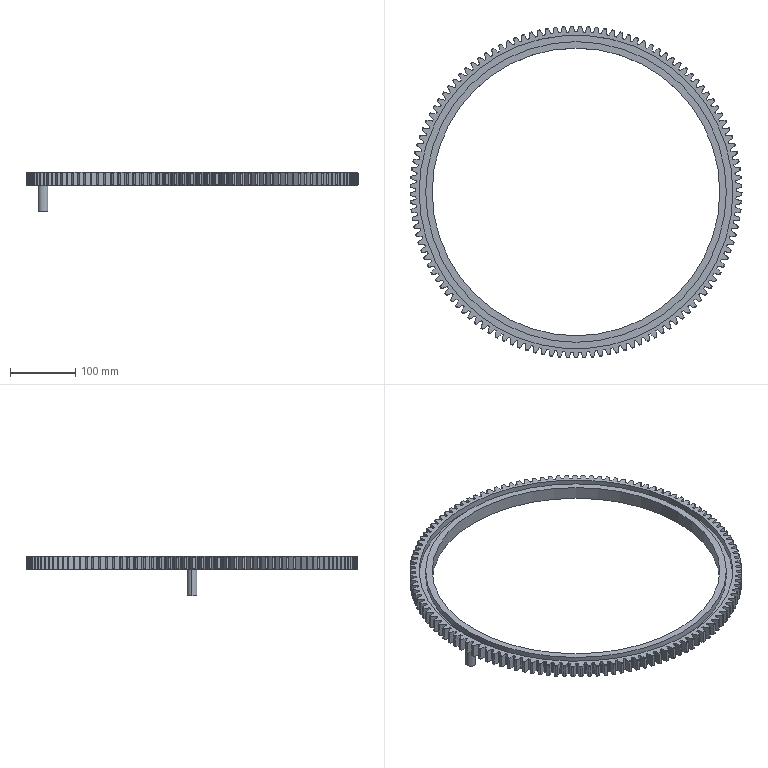Part | SolidWorks | 1 solid | 1064 faces | box 507.991 x 507.957 x 60 mm | volume 736026 mm3 | cylinder 559 | cone 250 | spline 250 | plane 5 | commonest cylinder face diameters 0.6 x301 490 x125 508 x125 15 x2 440 x2 460 x2